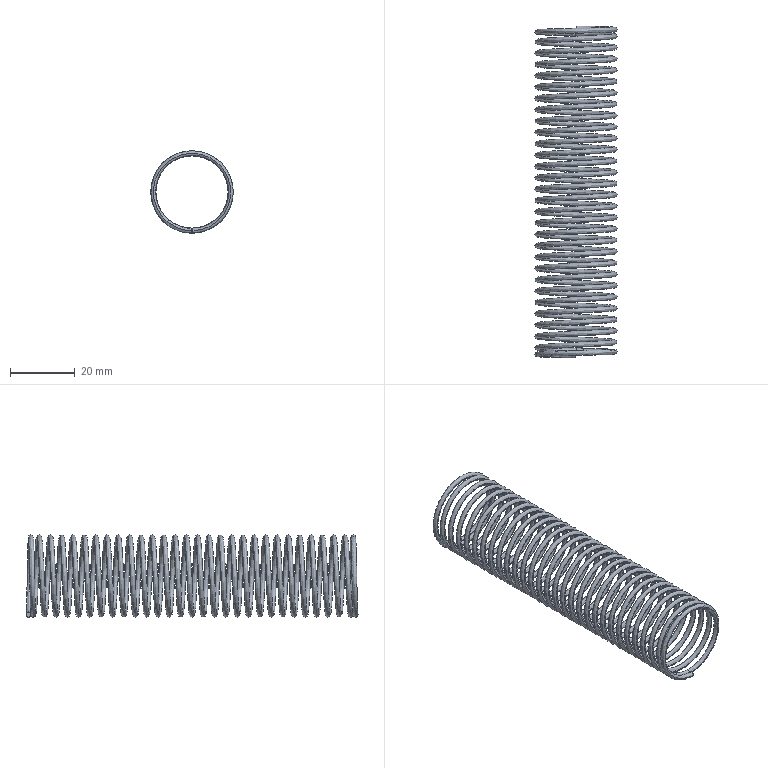Part | STEP file | 101000007777 | 1 solid | 8 faces | box 25.4 x 102.52 x 25.4 mm | volume 3984 mm3 | spline 6 | plane 2